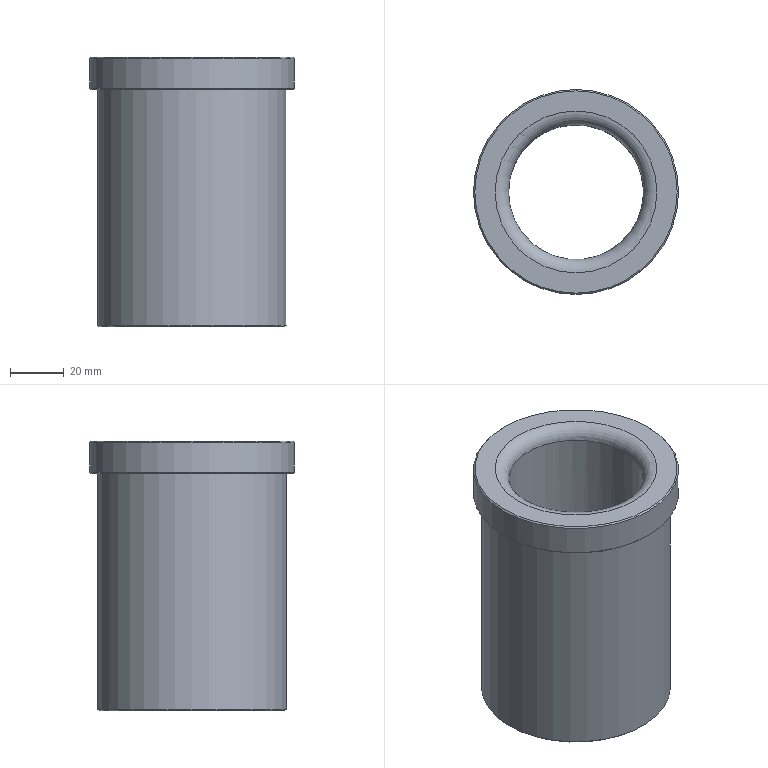Part | NX | features 模具.stp<1>[43] 2 | 1 solid | 11 faces | box 76 x 76 x 100 mm | volume 194904 mm3 | cylinder 3 | cone 3 | plane 3 | torus 2 | commonest cylinder face diameters 50 x1 70 x1 76 x1
STEP:
#1=CARTESIAN_POINT('',(217.,-295.,5.5));
#2=VERTEX_POINT('',#1);
#3=CARTESIAN_POINT('',(247.,-295.,5.5));
#4=DIRECTION('',(0.,0.,1.));
#5=DIRECTION('',(-1.,0.,0.));
#6=AXIS2_PLACEMENT_3D('',#3,#4,#5);
#7=CIRCLE('',#6,30.);
#8=EDGE_CURVE('',#2,#2,#7,.T.);
#9=ORIENTED_EDGE('',*,*,#8,.F.);
#10=EDGE_LOOP('',(#9));
#11=FACE_BOUND('',#10,.T.);
#12=CARTESIAN_POINT('',(222.,-295.,10.5));
#13=VERTEX_POINT('',#12);
#14=CARTESIAN_POINT('',(247.,-295.,10.5));
#15=DIRECTION('',(0.,0.,-1.));
#16=DIRECTION('',(-1.,0.,0.));
#17=AXIS2_PLACEMENT_3D('',#14,#15,#16);
#18=CIRCLE('',#17,25.);
#19=EDGE_CURVE('',#13,#13,#18,.T.);
#20=ORIENTED_EDGE('',*,*,#19,.F.);
#21=EDGE_LOOP('',(#20));
#22=FACE_BOUND('',#21,.T.);
#23=CARTESIAN_POINT('',(247.,-295.,10.5));
#24=DIRECTION('',(0.,0.,-1.));
#25=DIRECTION('',(-1.,0.,0.));
#26=AXIS2_PLACEMENT_3D('',#23,#24,#25);
#27=TOROIDAL_SURFACE('',#26,30.,5.);
#28=ADVANCED_FACE('',(#11,#22),#27,.T.);
#29=CARTESIAN_POINT('',(277.,-295.,105.5));
#30=VERTEX_POINT('',#29);
#31=CARTESIAN_POINT('',(247.,-295.,105.5));
#32=DIRECTION('',(0.,0.,-1.));
#33=DIRECTION('',(1.,0.,0.));
#34=AXIS2_PLACEMENT_3D('',#31,#32,#33);
#35=CIRCLE('',#34,30.);
#36=EDGE_CURVE('',#30,#30,#35,.T.);
#37=ORIENTED_EDGE('',*,*,#36,.F.);
#38=EDGE_LOOP('',(#37));
#39=FACE_BOUND('',#38,.T.);
#40=CARTESIAN_POINT('',(272.,-295.,100.5));
#41=VERTEX_POINT('',#40);
#42=CARTESIAN_POINT('',(247.,-295.,100.5));
#43=DIRECTION('',(0.,0.,1.));
#44=DIRECTION('',(1.,0.,0.));
#45=AXIS2_PLACEMENT_3D('',#42,#43,#44);
#46=CIRCLE('',#45,25.);
#47=EDGE_CURVE('',#41,#41,#46,.T.);
#48=ORIENTED_EDGE('',*,*,#47,.F.);
#49=EDGE_LOOP('',(#48));
#50=FACE_BOUND('',#49,.T.);
#51=CARTESIAN_POINT('',(247.,-295.,100.5));
#52=DIRECTION('',(0.,0.,1.));
#53=DIRECTION('',(1.,0.,0.));
#54=AXIS2_PLACEMENT_3D('',#51,#52,#53);
#55=TOROIDAL_SURFACE('',#54,30.,5.);
#56=ADVANCED_FACE('',(#39,#50),#55,.T.);
#57=ORIENTED_EDGE('',*,*,#19,.T.);
#58=EDGE_LOOP('',(#57));
#59=FACE_BOUND('',#58,.T.);
#60=ORIENTED_EDGE('',*,*,#47,.T.);
#61=EDGE_LOOP('',(#60));
#62=FACE_BOUND('',#61,.T.);
#63=CARTESIAN_POINT('',(247.,-295.,105.5));
#64=DIRECTION('',(0.,0.,-1.));
#65=DIRECTION('',(-1.,0.,0.));
#66=AXIS2_PLACEMENT_3D('',#63,#64,#65);
#67=CYLINDRICAL_SURFACE('',#66,25.);
#68=ADVANCED_FACE('',(#59,#62),#67,.F.);
#69=CARTESIAN_POINT('',(212.,-295.,6.));
#70=VERTEX_POINT('',#69);
#71=CARTESIAN_POINT('',(247.,-295.,6.));
#72=DIRECTION('',(0.,0.,1.));
#73=DIRECTION('',(-1.,0.,0.));
#74=AXIS2_PLACEMENT_3D('',#71,#72,#73);
#75=CIRCLE('',#74,35.);
#76=EDGE_CURVE('',#70,#70,#75,.T.);
#77=ORIENTED_EDGE('',*,*,#76,.F.);
#78=EDGE_LOOP('',(#77));
#79=FACE_BOUND('',#78,.T.);
#80=CARTESIAN_POINT('',(212.5,-295.,5.5));
#81=VERTEX_POINT('',#80);
#82=CARTESIAN_POINT('',(247.,-295.,5.5));
#83=DIRECTION('',(0.,0.,-1.));
#84=DIRECTION('',(-1.,0.,0.));
#85=AXIS2_PLACEMENT_3D('',#82,#83,#84);
#86=CIRCLE('',#85,34.5);
#87=EDGE_CURVE('',#81,#81,#86,.T.);
#88=ORIENTED_EDGE('',*,*,#87,.F.);
#89=EDGE_LOOP('',(#88));
#90=FACE_BOUND('',#89,.T.);
#91=CARTESIAN_POINT('',(247.,-295.,6.));
#92=DIRECTION('',(0.,0.,1.));
#93=DIRECTION('',(1.,0.,0.));
#94=AXIS2_PLACEMENT_3D('',#91,#92,#93);
#95=CONICAL_SURFACE('',#94,35.,0.7854);
#96=ADVANCED_FACE('',(#79,#90),#95,.T.);
#97=ORIENTED_EDGE('',*,*,#76,.T.);
#98=EDGE_LOOP('',(#97));
#99=FACE_BOUND('',#98,.T.);
#100=CARTESIAN_POINT('',(212.,-295.,93.5));
#101=VERTEX_POINT('',#100);
#102=CARTESIAN_POINT('',(247.,-295.,93.5));
#103=DIRECTION('',(0.,0.,-1.));
#104=DIRECTION('',(-1.,0.,0.));
#105=AXIS2_PLACEMENT_3D('',#102,#103,#104);
#106=CIRCLE('',#105,35.);
#107=EDGE_CURVE('',#101,#101,#106,.T.);
#108=ORIENTED_EDGE('',*,*,#107,.T.);
#109=EDGE_LOOP('',(#108));
#110=FACE_BOUND('',#109,.T.);
#111=CARTESIAN_POINT('',(247.,-295.,105.5));
#112=DIRECTION('',(0.,0.,-1.));
#113=DIRECTION('',(-1.,0.,0.));
#114=AXIS2_PLACEMENT_3D('',#111,#112,#113);
#115=CYLINDRICAL_SURFACE('',#114,35.);
#116=ADVANCED_FACE('',(#99,#110),#115,.T.);
#117=ORIENTED_EDGE('',*,*,#87,.T.);
#118=EDGE_LOOP('',(#117));
#119=FACE_BOUND('',#118,.T.);
#120=ORIENTED_EDGE('',*,*,#8,.T.);
#121=EDGE_LOOP('',(#120));
#122=FACE_BOUND('',#121,.T.);
#123=CARTESIAN_POINT('',(247.,-295.,5.5));
#124=DIRECTION('',(0.,0.,-1.));
#125=DIRECTION('',(0.,-1.,0.));
#126=AXIS2_PLACEMENT_3D('',#123,#124,#125);
#127=PLANE('',#126);
#128=ADVANCED_FACE('',(#119,#122),#127,.T.);
#129=CARTESIAN_POINT('',(209.,-295.,94.));
#130=VERTEX_POINT('',#129);
#131=CARTESIAN_POINT('',(247.,-295.,94.));
#132=DIRECTION('',(0.,0.,1.));
#133=DIRECTION('',(-1.,0.,0.));
#134=AXIS2_PLACEMENT_3D('',#131,#132,#133);
#135=CIRCLE('',#134,38.);
#136=EDGE_CURVE('',#130,#130,#135,.T.);
#137=ORIENTED_EDGE('',*,*,#136,.F.);
#138=EDGE_LOOP('',(#137));
#139=FACE_BOUND('',#138,.T.);
#140=CARTESIAN_POINT('',(209.5,-295.,93.5));
#141=VERTEX_POINT('',#140);
#142=CARTESIAN_POINT('',(247.,-295.,93.5));
#143=DIRECTION('',(0.,0.,-1.));
#144=DIRECTION('',(-1.,0.,0.));
#145=AXIS2_PLACEMENT_3D('',#142,#143,#144);
#146=CIRCLE('',#145,37.5);
#147=EDGE_CURVE('',#141,#141,#146,.T.);
#148=ORIENTED_EDGE('',*,*,#147,.F.);
#149=EDGE_LOOP('',(#148));
#150=FACE_BOUND('',#149,.T.);
#151=CARTESIAN_POINT('',(247.,-295.,94.));
#152=DIRECTION('',(0.,0.,1.));
#153=DIRECTION('',(1.,0.,0.));
#154=AXIS2_PLACEMENT_3D('',#151,#152,#153);
#155=CONICAL_SURFACE('',#154,38.,0.7854);
#156=ADVANCED_FACE('',(#139,#150),#155,.T.);
#157=CARTESIAN_POINT('',(285.,-295.,105.));
#158=VERTEX_POINT('',#157);
#159=CARTESIAN_POINT('',(247.,-295.,105.));
#160=DIRECTION('',(0.,0.,-1.));
#161=DIRECTION('',(1.,0.,0.));
#162=AXIS2_PLACEMENT_3D('',#159,#160,#161);
#163=CIRCLE('',#162,38.);
#164=EDGE_CURVE('',#158,#158,#163,.T.);
#165=ORIENTED_EDGE('',*,*,#164,.F.);
#166=EDGE_LOOP('',(#165));
#167=FACE_BOUND('',#166,.T.);
#168=CARTESIAN_POINT('',(284.5,-295.,105.5));
#169=VERTEX_POINT('',#168);
#170=CARTESIAN_POINT('',(247.,-295.,105.5));
#171=DIRECTION('',(0.,0.,1.));
#172=DIRECTION('',(1.,0.,0.));
#173=AXIS2_PLACEMENT_3D('',#170,#171,#172);
#174=CIRCLE('',#173,37.5);
#175=EDGE_CURVE('',#169,#169,#174,.T.);
#176=ORIENTED_EDGE('',*,*,#175,.F.);
#177=EDGE_LOOP('',(#176));
#178=FACE_BOUND('',#177,.T.);
#179=CARTESIAN_POINT('',(247.,-295.,105.));
#180=DIRECTION('',(0.,0.,-1.));
#181=DIRECTION('',(-1.,0.,0.));
#182=AXIS2_PLACEMENT_3D('',#179,#180,#181);
#183=CONICAL_SURFACE('',#182,38.,0.7854);
#184=ADVANCED_FACE('',(#167,#178),#183,.T.);
#185=ORIENTED_EDGE('',*,*,#136,.T.);
#186=EDGE_LOOP('',(#185));
#187=FACE_BOUND('',#186,.T.);
#188=ORIENTED_EDGE('',*,*,#164,.T.);
#189=EDGE_LOOP('',(#188));
#190=FACE_BOUND('',#189,.T.);
#191=CARTESIAN_POINT('',(247.,-295.,105.5));
#192=DIRECTION('',(0.,0.,-1.));
#193=DIRECTION('',(-1.,0.,0.));
#194=AXIS2_PLACEMENT_3D('',#191,#192,#193);
#195=CYLINDRICAL_SURFACE('',#194,38.);
#196=ADVANCED_FACE('',(#187,#190),#195,.T.);
#197=ORIENTED_EDGE('',*,*,#36,.T.);
#198=EDGE_LOOP('',(#197));
#199=FACE_BOUND('',#198,.T.);
#200=ORIENTED_EDGE('',*,*,#175,.T.);
#201=EDGE_LOOP('',(#200));
#202=FACE_BOUND('',#201,.T.);
#203=CARTESIAN_POINT('',(247.,-295.,105.5));
#204=DIRECTION('',(0.,0.,1.));
#205=DIRECTION('',(1.,0.,0.));
#206=AXIS2_PLACEMENT_3D('',#203,#204,#205);
#207=PLANE('',#206);
#208=ADVANCED_FACE('',(#199,#202),#207,.T.);
#209=ORIENTED_EDGE('',*,*,#147,.T.);
#210=EDGE_LOOP('',(#209));
#211=FACE_BOUND('',#210,.T.);
#212=ORIENTED_EDGE('',*,*,#107,.F.);
#213=EDGE_LOOP('',(#212));
#214=FACE_BOUND('',#213,.T.);
#215=CARTESIAN_POINT('',(247.,-295.,93.5));
#216=DIRECTION('',(0.,0.,-1.));
#217=DIRECTION('',(0.,-1.,0.));
#218=AXIS2_PLACEMENT_3D('',#215,#216,#217);
#219=PLANE('',#218);
#220=ADVANCED_FACE('',(#211,#214),#219,.T.);
#221=CLOSED_SHELL('',(#28,#56,#68,#96,#116,#128,#156,#184,#196,#208,#220));
#222=MANIFOLD_SOLID_BREP('',#221);
#223=(LENGTH_UNIT()NAMED_UNIT(*)SI_UNIT(.MILLI.,.METRE.));
#224=UNCERTAINTY_MEASURE_WITH_UNIT(LENGTH_MEASURE(0.00001),#223,'','');
#225=(NAMED_UNIT(*)PLANE_ANGLE_UNIT()SI_UNIT($,.RADIAN.));
#226=(NAMED_UNIT(*)SI_UNIT($,.STERADIAN.)SOLID_ANGLE_UNIT());
#227=(GEOMETRIC_REPRESENTATION_CONTEXT(3)GLOBAL_UNCERTAINTY_ASSIGNED_CONTEXT((#224))GLOBAL_UNIT_ASSIGNED_CONTEXT((#223,#225,#226))REPRESENTATION_CONTEXT('',''));
#228=ADVANCED_BREP_SHAPE_REPRESENTATION('',(#222),#227);